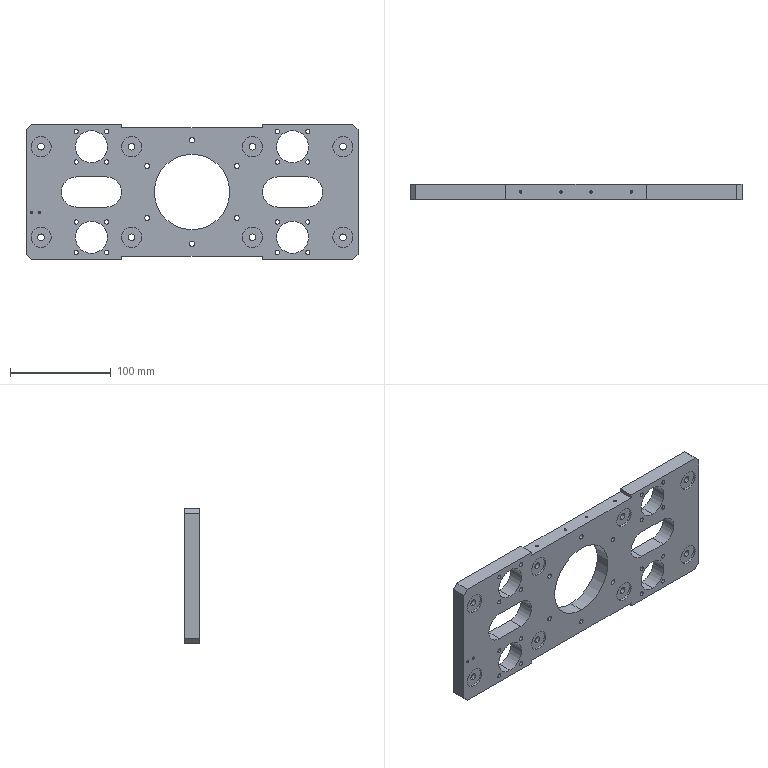Part | SolidWorks | features BaseBody 1 | 1 solid | 192 faces | box 330 x 15 x 135 mm | volume 472507 mm3 | cylinder 130 | plane 38 | cone 24 | commonest cylinder face diameters 4.2 x32 2.5 x20 6.6 x16 11 x16 20 x16 5 x12